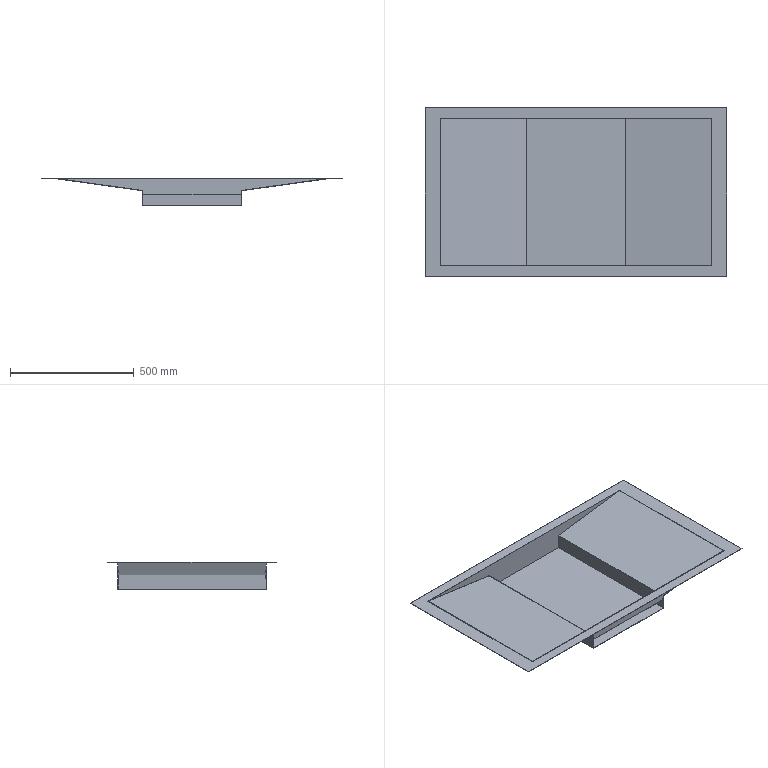Part | STEP file | HJDX-305 | 1 solid | 23 faces | box 1220 x 680 x 110 mm | volume 1513964 mm3 | plane 23
STEP:
#1=CARTESIAN_POINT('',(-200.,-300.,0.));
#2=VERTEX_POINT('',#1);
#3=CARTESIAN_POINT('',(-200.,300.,0.));
#4=VERTEX_POINT('',#3);
#5=CARTESIAN_POINT('',(-200.,0.,0.));
#6=DIRECTION('',(0.,1.,0.));
#7=VECTOR('',#6,1000.);
#8=LINE('',#5,#7);
#9=EDGE_CURVE('',#2,#4,#8,.T.);
#10=ORIENTED_EDGE('',*,*,#9,.T.);
#11=CARTESIAN_POINT('',(200.,300.,0.));
#12=VERTEX_POINT('',#11);
#13=CARTESIAN_POINT('',(0.,300.,0.));
#14=DIRECTION('',(1.,0.,0.));
#15=VECTOR('',#14,1000.);
#16=LINE('',#13,#15);
#17=EDGE_CURVE('',#4,#12,#16,.T.);
#18=ORIENTED_EDGE('',*,*,#17,.T.);
#19=CARTESIAN_POINT('',(200.,-300.,0.));
#20=VERTEX_POINT('',#19);
#21=CARTESIAN_POINT('',(200.,0.,0.));
#22=DIRECTION('',(0.,-1.,0.));
#23=VECTOR('',#22,1000.);
#24=LINE('',#21,#23);
#25=EDGE_CURVE('',#12,#20,#24,.T.);
#26=ORIENTED_EDGE('',*,*,#25,.T.);
#27=CARTESIAN_POINT('',(0.,-300.,0.));
#28=DIRECTION('',(-1.,0.,0.));
#29=VECTOR('',#28,1000.);
#30=LINE('',#27,#29);
#31=EDGE_CURVE('',#20,#2,#30,.T.);
#32=ORIENTED_EDGE('',*,*,#31,.T.);
#33=EDGE_LOOP('',(#10,#18,#26,#32));
#34=FACE_OUTER_BOUND('',#33,.T.);
#35=CARTESIAN_POINT('',(0.,0.,0.));
#36=DIRECTION('',(0.,0.,-1.));
#37=DIRECTION('',(-1.,0.,0.));
#38=AXIS2_PLACEMENT_3D('',#35,#36,#37);
#39=PLANE('',#38);
#40=ADVANCED_FACE('',(#34),#39,.T.);
#41=CARTESIAN_POINT('',(550.,300.,108.5));
#42=VERTEX_POINT('',#41);
#43=CARTESIAN_POINT('',(-550.,300.,108.5));
#44=VERTEX_POINT('',#43);
#45=CARTESIAN_POINT('',(-200.,300.,108.5));
#46=DIRECTION('',(-1.,0.,0.));
#47=VECTOR('',#46,1000.);
#48=LINE('',#45,#47);
#49=EDGE_CURVE('',#42,#44,#48,.T.);
#50=ORIENTED_EDGE('',*,*,#49,.F.);
#51=CARTESIAN_POINT('',(200.,300.,60.));
#52=VERTEX_POINT('',#51);
#53=CARTESIAN_POINT('',(200.,300.,60.));
#54=DIRECTION('',(0.9905,0.,0.1373));
#55=VECTOR('',#54,1000.);
#56=LINE('',#53,#55);
#57=EDGE_CURVE('',#52,#42,#56,.T.);
#58=ORIENTED_EDGE('',*,*,#57,.F.);
#59=CARTESIAN_POINT('',(200.,300.,60.));
#60=DIRECTION('',(0.,0.,1.));
#61=VECTOR('',#60,1000.);
#62=LINE('',#59,#61);
#63=EDGE_CURVE('',#12,#52,#62,.T.);
#64=ORIENTED_EDGE('',*,*,#63,.F.);
#65=ORIENTED_EDGE('',*,*,#17,.F.);
#66=CARTESIAN_POINT('',(-200.,300.,60.));
#67=VERTEX_POINT('',#66);
#68=CARTESIAN_POINT('',(-200.,300.,60.));
#69=DIRECTION('',(0.,0.,-1.));
#70=VECTOR('',#69,1000.);
#71=LINE('',#68,#70);
#72=EDGE_CURVE('',#67,#4,#71,.T.);
#73=ORIENTED_EDGE('',*,*,#72,.F.);
#74=CARTESIAN_POINT('',(-550.,300.,108.5));
#75=DIRECTION('',(0.9905,0.,-0.1373));
#76=VECTOR('',#75,1000.);
#77=LINE('',#74,#76);
#78=EDGE_CURVE('',#44,#67,#77,.T.);
#79=ORIENTED_EDGE('',*,*,#78,.F.);
#80=EDGE_LOOP('',(#50,#58,#64,#65,#73,#79));
#81=FACE_OUTER_BOUND('',#80,.T.);
#82=CARTESIAN_POINT('',(-200.,300.,60.));
#83=DIRECTION('',(0.,-1.,0.));
#84=DIRECTION('',(0.,0.,-1.));
#85=AXIS2_PLACEMENT_3D('',#82,#83,#84);
#86=PLANE('',#85);
#87=ADVANCED_FACE('',(#81),#86,.F.);
#88=CARTESIAN_POINT('',(-200.,-300.,60.));
#89=VERTEX_POINT('',#88);
#90=CARTESIAN_POINT('',(-200.,-300.,60.));
#91=DIRECTION('',(0.,0.,-1.));
#92=VECTOR('',#91,1000.);
#93=LINE('',#90,#92);
#94=EDGE_CURVE('',#89,#2,#93,.T.);
#95=ORIENTED_EDGE('',*,*,#94,.F.);
#96=CARTESIAN_POINT('',(-200.,-300.,60.));
#97=DIRECTION('',(0.,-1.,0.));
#98=VECTOR('',#97,1000.);
#99=LINE('',#96,#98);
#100=EDGE_CURVE('',#67,#89,#99,.T.);
#101=ORIENTED_EDGE('',*,*,#100,.F.);
#102=ORIENTED_EDGE('',*,*,#72,.T.);
#103=ORIENTED_EDGE('',*,*,#9,.F.);
#104=EDGE_LOOP('',(#95,#101,#102,#103));
#105=FACE_OUTER_BOUND('',#104,.T.);
#106=CARTESIAN_POINT('',(-200.,-300.,60.));
#107=DIRECTION('',(1.,0.,0.));
#108=DIRECTION('',(0.,0.,-1.));
#109=AXIS2_PLACEMENT_3D('',#106,#107,#108);
#110=PLANE('',#109);
#111=ADVANCED_FACE('',(#105),#110,.F.);
#112=CARTESIAN_POINT('',(-550.,-300.,108.5));
#113=VERTEX_POINT('',#112);
#114=CARTESIAN_POINT('',(550.,-300.,108.5));
#115=VERTEX_POINT('',#114);
#116=CARTESIAN_POINT('',(-200.,-300.,108.5));
#117=DIRECTION('',(1.,0.,0.));
#118=VECTOR('',#117,1000.);
#119=LINE('',#116,#118);
#120=EDGE_CURVE('',#113,#115,#119,.T.);
#121=ORIENTED_EDGE('',*,*,#120,.F.);
#122=CARTESIAN_POINT('',(-200.,-300.,60.));
#123=DIRECTION('',(-0.9905,0.,0.1373));
#124=VECTOR('',#123,1000.);
#125=LINE('',#122,#124);
#126=EDGE_CURVE('',#89,#113,#125,.T.);
#127=ORIENTED_EDGE('',*,*,#126,.F.);
#128=ORIENTED_EDGE('',*,*,#94,.T.);
#129=ORIENTED_EDGE('',*,*,#31,.F.);
#130=CARTESIAN_POINT('',(200.,-300.,60.));
#131=VERTEX_POINT('',#130);
#132=CARTESIAN_POINT('',(200.,-300.,60.));
#133=DIRECTION('',(0.,0.,-1.));
#134=VECTOR('',#133,1000.);
#135=LINE('',#132,#134);
#136=EDGE_CURVE('',#131,#20,#135,.T.);
#137=ORIENTED_EDGE('',*,*,#136,.F.);
#138=CARTESIAN_POINT('',(550.,-300.,108.5));
#139=DIRECTION('',(-0.9905,0.,-0.1373));
#140=VECTOR('',#139,1000.);
#141=LINE('',#138,#140);
#142=EDGE_CURVE('',#115,#131,#141,.T.);
#143=ORIENTED_EDGE('',*,*,#142,.F.);
#144=EDGE_LOOP('',(#121,#127,#128,#129,#137,#143));
#145=FACE_OUTER_BOUND('',#144,.T.);
#146=CARTESIAN_POINT('',(198.5,-300.,1.5));
#147=VERTEX_POINT('',#146);
#148=CARTESIAN_POINT('',(198.5,-300.,43.5));
#149=VERTEX_POINT('',#148);
#150=CARTESIAN_POINT('',(198.5,-300.,60.));
#151=DIRECTION('',(0.,0.,1.));
#152=VECTOR('',#151,1000.);
#153=LINE('',#150,#152);
#154=EDGE_CURVE('',#147,#149,#153,.T.);
#155=ORIENTED_EDGE('',*,*,#154,.F.);
#156=CARTESIAN_POINT('',(-198.5,-300.,1.5));
#157=VERTEX_POINT('',#156);
#158=CARTESIAN_POINT('',(-200.,-300.,1.5));
#159=DIRECTION('',(1.,0.,0.));
#160=VECTOR('',#159,1000.);
#161=LINE('',#158,#160);
#162=EDGE_CURVE('',#157,#147,#161,.T.);
#163=ORIENTED_EDGE('',*,*,#162,.F.);
#164=CARTESIAN_POINT('',(-198.5,-300.,43.5));
#165=VERTEX_POINT('',#164);
#166=CARTESIAN_POINT('',(-198.5,-300.,60.));
#167=DIRECTION('',(0.,0.,-1.));
#168=VECTOR('',#167,1000.);
#169=LINE('',#166,#168);
#170=EDGE_CURVE('',#165,#157,#169,.T.);
#171=ORIENTED_EDGE('',*,*,#170,.F.);
#172=CARTESIAN_POINT('',(-200.,-300.,43.5));
#173=DIRECTION('',(-1.,0.,0.));
#174=VECTOR('',#173,1000.);
#175=LINE('',#172,#174);
#176=EDGE_CURVE('',#149,#165,#175,.T.);
#177=ORIENTED_EDGE('',*,*,#176,.F.);
#178=EDGE_LOOP('',(#155,#163,#171,#177));
#179=FACE_BOUND('',#178,.T.);
#180=CARTESIAN_POINT('',(-200.,-300.,60.));
#181=DIRECTION('',(0.,1.,0.));
#182=DIRECTION('',(0.,0.,1.));
#183=AXIS2_PLACEMENT_3D('',#180,#181,#182);
#184=PLANE('',#183);
#185=ADVANCED_FACE('',(#145,#179),#184,.F.);
#186=ORIENTED_EDGE('',*,*,#63,.T.);
#187=CARTESIAN_POINT('',(200.,-300.,60.));
#188=DIRECTION('',(0.,1.,0.));
#189=VECTOR('',#188,1000.);
#190=LINE('',#187,#189);
#191=EDGE_CURVE('',#131,#52,#190,.T.);
#192=ORIENTED_EDGE('',*,*,#191,.F.);
#193=ORIENTED_EDGE('',*,*,#136,.T.);
#194=ORIENTED_EDGE('',*,*,#25,.F.);
#195=EDGE_LOOP('',(#186,#192,#193,#194));
#196=FACE_OUTER_BOUND('',#195,.T.);
#197=CARTESIAN_POINT('',(200.,-300.,60.));
#198=DIRECTION('',(-1.,0.,0.));
#199=DIRECTION('',(0.,0.,1.));
#200=AXIS2_PLACEMENT_3D('',#197,#198,#199);
#201=PLANE('',#200);
#202=ADVANCED_FACE('',(#196),#201,.F.);
#203=CARTESIAN_POINT('',(-550.,300.,108.5));
#204=DIRECTION('',(0.,-1.,0.));
#205=VECTOR('',#204,1000.);
#206=LINE('',#203,#205);
#207=EDGE_CURVE('',#44,#113,#206,.T.);
#208=ORIENTED_EDGE('',*,*,#207,.F.);
#209=ORIENTED_EDGE('',*,*,#78,.T.);
#210=ORIENTED_EDGE('',*,*,#100,.T.);
#211=ORIENTED_EDGE('',*,*,#126,.T.);
#212=EDGE_LOOP('',(#208,#209,#210,#211));
#213=FACE_OUTER_BOUND('',#212,.T.);
#214=CARTESIAN_POINT('',(-550.,300.,108.5));
#215=DIRECTION('',(0.1373,0.,0.9905));
#216=DIRECTION('',(0.9905,0.,-0.1373));
#217=AXIS2_PLACEMENT_3D('',#214,#215,#216);
#218=PLANE('',#217);
#219=ADVANCED_FACE('',(#213),#218,.F.);
#220=CARTESIAN_POINT('',(-610.,-340.,108.5));
#221=VERTEX_POINT('',#220);
#222=CARTESIAN_POINT('',(-610.,340.,108.5));
#223=VERTEX_POINT('',#222);
#224=CARTESIAN_POINT('',(-610.,0.,108.5));
#225=DIRECTION('',(0.,1.,0.));
#226=VECTOR('',#225,1000.);
#227=LINE('',#224,#226);
#228=EDGE_CURVE('',#221,#223,#227,.T.);
#229=ORIENTED_EDGE('',*,*,#228,.T.);
#230=CARTESIAN_POINT('',(610.,340.,108.5));
#231=VERTEX_POINT('',#230);
#232=CARTESIAN_POINT('',(0.,340.,108.5));
#233=DIRECTION('',(1.,0.,0.));
#234=VECTOR('',#233,1000.);
#235=LINE('',#232,#234);
#236=EDGE_CURVE('',#223,#231,#235,.T.);
#237=ORIENTED_EDGE('',*,*,#236,.T.);
#238=CARTESIAN_POINT('',(610.,-340.,108.5));
#239=VERTEX_POINT('',#238);
#240=CARTESIAN_POINT('',(610.,0.,108.5));
#241=DIRECTION('',(0.,-1.,0.));
#242=VECTOR('',#241,1000.);
#243=LINE('',#240,#242);
#244=EDGE_CURVE('',#231,#239,#243,.T.);
#245=ORIENTED_EDGE('',*,*,#244,.T.);
#246=CARTESIAN_POINT('',(0.,-340.,108.5));
#247=DIRECTION('',(-1.,0.,0.));
#248=VECTOR('',#247,1000.);
#249=LINE('',#246,#248);
#250=EDGE_CURVE('',#239,#221,#249,.T.);
#251=ORIENTED_EDGE('',*,*,#250,.T.);
#252=EDGE_LOOP('',(#229,#237,#245,#251));
#253=FACE_OUTER_BOUND('',#252,.T.);
#254=ORIENTED_EDGE('',*,*,#207,.T.);
#255=ORIENTED_EDGE('',*,*,#120,.T.);
#256=CARTESIAN_POINT('',(550.,0.,108.5));
#257=DIRECTION('',(0.,1.,0.));
#258=VECTOR('',#257,1000.);
#259=LINE('',#256,#258);
#260=EDGE_CURVE('',#115,#42,#259,.T.);
#261=ORIENTED_EDGE('',*,*,#260,.T.);
#262=ORIENTED_EDGE('',*,*,#49,.T.);
#263=EDGE_LOOP('',(#254,#255,#261,#262));
#264=FACE_BOUND('',#263,.T.);
#265=CARTESIAN_POINT('',(0.,0.,108.5));
#266=DIRECTION('',(0.,0.,-1.));
#267=DIRECTION('',(-1.,0.,0.));
#268=AXIS2_PLACEMENT_3D('',#265,#266,#267);
#269=PLANE('',#268);
#270=ADVANCED_FACE('',(#253,#264),#269,.T.);
#271=ORIENTED_EDGE('',*,*,#191,.T.);
#272=ORIENTED_EDGE('',*,*,#57,.T.);
#273=ORIENTED_EDGE('',*,*,#260,.F.);
#274=ORIENTED_EDGE('',*,*,#142,.T.);
#275=EDGE_LOOP('',(#271,#272,#273,#274));
#276=FACE_OUTER_BOUND('',#275,.T.);
#277=CARTESIAN_POINT('',(200.,300.,60.));
#278=DIRECTION('',(-0.1373,0.,0.9905));
#279=DIRECTION('',(0.9905,0.,0.1373));
#280=AXIS2_PLACEMENT_3D('',#277,#278,#279);
#281=PLANE('',#280);
#282=ADVANCED_FACE('',(#276),#281,.F.);
#283=CARTESIAN_POINT('',(198.5,-298.5,43.5));
#284=VERTEX_POINT('',#283);
#285=CARTESIAN_POINT('',(198.5,697.715,43.5));
#286=DIRECTION('',(0.,1.,0.));
#287=VECTOR('',#286,1000.);
#288=LINE('',#285,#287);
#289=EDGE_CURVE('',#149,#284,#288,.T.);
#290=ORIENTED_EDGE('',*,*,#289,.F.);
#291=ORIENTED_EDGE('',*,*,#176,.T.);
#292=CARTESIAN_POINT('',(-198.5,-298.5,43.5));
#293=VERTEX_POINT('',#292);
#294=CARTESIAN_POINT('',(-198.5,697.715,43.5));
#295=DIRECTION('',(0.,-1.,0.));
#296=VECTOR('',#295,1000.);
#297=LINE('',#294,#296);
#298=EDGE_CURVE('',#293,#165,#297,.T.);
#299=ORIENTED_EDGE('',*,*,#298,.F.);
#300=CARTESIAN_POINT('',(-198.5,-298.5,43.5));
#301=DIRECTION('',(-1.,0.,0.));
#302=VECTOR('',#301,1000.);
#303=LINE('',#300,#302);
#304=EDGE_CURVE('',#284,#293,#303,.T.);
#305=ORIENTED_EDGE('',*,*,#304,.F.);
#306=EDGE_LOOP('',(#290,#291,#299,#305));
#307=FACE_OUTER_BOUND('',#306,.T.);
#308=CARTESIAN_POINT('',(-198.5,697.715,43.5));
#309=DIRECTION('',(0.,0.,1.));
#310=DIRECTION('',(1.,0.,0.));
#311=AXIS2_PLACEMENT_3D('',#308,#309,#310);
#312=PLANE('',#311);
#313=ADVANCED_FACE('',(#307),#312,.F.);
#314=CARTESIAN_POINT('',(198.5,-298.5,61.306));
#315=VERTEX_POINT('',#314);
#316=CARTESIAN_POINT('',(198.5,-298.5,60.));
#317=DIRECTION('',(0.,0.,1.));
#318=VECTOR('',#317,1000.);
#319=LINE('',#316,#318);
#320=EDGE_CURVE('',#284,#315,#319,.T.);
#321=ORIENTED_EDGE('',*,*,#320,.T.);
#322=CARTESIAN_POINT('',(198.5,298.5,61.306));
#323=VERTEX_POINT('',#322);
#324=CARTESIAN_POINT('',(198.5,-300.,61.306));
#325=DIRECTION('',(0.,1.,0.));
#326=VECTOR('',#325,1000.);
#327=LINE('',#324,#326);
#328=EDGE_CURVE('',#315,#323,#327,.T.);
#329=ORIENTED_EDGE('',*,*,#328,.T.);
#330=CARTESIAN_POINT('',(198.5,298.5,1.5));
#331=VERTEX_POINT('',#330);
#332=CARTESIAN_POINT('',(198.5,298.5,60.));
#333=DIRECTION('',(0.,0.,-1.));
#334=VECTOR('',#333,1000.);
#335=LINE('',#332,#334);
#336=EDGE_CURVE('',#323,#331,#335,.T.);
#337=ORIENTED_EDGE('',*,*,#336,.T.);
#338=CARTESIAN_POINT('',(198.5,-300.,1.5));
#339=DIRECTION('',(0.,-1.,0.));
#340=VECTOR('',#339,1000.);
#341=LINE('',#338,#340);
#342=EDGE_CURVE('',#331,#147,#341,.T.);
#343=ORIENTED_EDGE('',*,*,#342,.T.);
#344=ORIENTED_EDGE('',*,*,#154,.T.);
#345=ORIENTED_EDGE('',*,*,#289,.T.);
#346=EDGE_LOOP('',(#321,#329,#337,#343,#344,#345));
#347=FACE_OUTER_BOUND('',#346,.T.);
#348=CARTESIAN_POINT('',(198.5,-300.,60.));
#349=DIRECTION('',(-1.,0.,0.));
#350=DIRECTION('',(0.,0.,1.));
#351=AXIS2_PLACEMENT_3D('',#348,#349,#350);
#352=PLANE('',#351);
#353=ADVANCED_FACE('',(#347),#352,.T.);
#354=CARTESIAN_POINT('',(-198.5,298.5,1.5));
#355=VERTEX_POINT('',#354);
#356=CARTESIAN_POINT('',(0.,298.5,1.5));
#357=DIRECTION('',(1.,0.,0.));
#358=VECTOR('',#357,1000.);
#359=LINE('',#356,#358);
#360=EDGE_CURVE('',#355,#331,#359,.T.);
#361=ORIENTED_EDGE('',*,*,#360,.F.);
#362=CARTESIAN_POINT('',(-198.5,0.,1.5));
#363=DIRECTION('',(0.,1.,0.));
#364=VECTOR('',#363,1000.);
#365=LINE('',#362,#364);
#366=EDGE_CURVE('',#157,#355,#365,.T.);
#367=ORIENTED_EDGE('',*,*,#366,.F.);
#368=ORIENTED_EDGE('',*,*,#162,.T.);
#369=ORIENTED_EDGE('',*,*,#342,.F.);
#370=EDGE_LOOP('',(#361,#367,#368,#369));
#371=FACE_OUTER_BOUND('',#370,.T.);
#372=CARTESIAN_POINT('',(0.,0.,1.5));
#373=DIRECTION('',(0.,0.,-1.));
#374=DIRECTION('',(-1.,0.,0.));
#375=AXIS2_PLACEMENT_3D('',#372,#373,#374);
#376=PLANE('',#375);
#377=ADVANCED_FACE('',(#371),#376,.F.);
#378=CARTESIAN_POINT('',(-198.5,298.5,61.306));
#379=VERTEX_POINT('',#378);
#380=CARTESIAN_POINT('',(-198.5,298.5,60.));
#381=DIRECTION('',(0.,0.,1.));
#382=VECTOR('',#381,1000.);
#383=LINE('',#380,#382);
#384=EDGE_CURVE('',#355,#379,#383,.T.);
#385=ORIENTED_EDGE('',*,*,#384,.T.);
#386=CARTESIAN_POINT('',(-198.5,-298.5,61.306));
#387=VERTEX_POINT('',#386);
#388=CARTESIAN_POINT('',(-198.5,-300.,61.306));
#389=DIRECTION('',(0.,-1.,0.));
#390=VECTOR('',#389,1000.);
#391=LINE('',#388,#390);
#392=EDGE_CURVE('',#379,#387,#391,.T.);
#393=ORIENTED_EDGE('',*,*,#392,.T.);
#394=CARTESIAN_POINT('',(-198.5,-298.5,60.));
#395=DIRECTION('',(0.,0.,-1.));
#396=VECTOR('',#395,1000.);
#397=LINE('',#394,#396);
#398=EDGE_CURVE('',#387,#293,#397,.T.);
#399=ORIENTED_EDGE('',*,*,#398,.T.);
#400=ORIENTED_EDGE('',*,*,#298,.T.);
#401=ORIENTED_EDGE('',*,*,#170,.T.);
#402=ORIENTED_EDGE('',*,*,#366,.T.);
#403=EDGE_LOOP('',(#385,#393,#399,#400,#401,#402));
#404=FACE_OUTER_BOUND('',#403,.T.);
#405=CARTESIAN_POINT('',(-198.5,-300.,60.));
#406=DIRECTION('',(1.,0.,0.));
#407=DIRECTION('',(0.,0.,-1.));
#408=AXIS2_PLACEMENT_3D('',#405,#406,#407);
#409=PLANE('',#408);
#410=ADVANCED_FACE('',(#404),#409,.T.);
#411=ORIENTED_EDGE('',*,*,#236,.F.);
#412=CARTESIAN_POINT('',(-610.,340.,110.));
#413=VERTEX_POINT('',#412);
#414=CARTESIAN_POINT('',(-610.,340.,108.5));
#415=DIRECTION('',(0.,0.,1.));
#416=VECTOR('',#415,1000.);
#417=LINE('',#414,#416);
#418=EDGE_CURVE('',#223,#413,#417,.T.);
#419=ORIENTED_EDGE('',*,*,#418,.T.);
#420=CARTESIAN_POINT('',(610.,340.,110.));
#421=VERTEX_POINT('',#420);
#422=CARTESIAN_POINT('',(-610.,340.,110.));
#423=DIRECTION('',(1.,0.,0.));
#424=VECTOR('',#423,1000.);
#425=LINE('',#422,#424);
#426=EDGE_CURVE('',#413,#421,#425,.T.);
#427=ORIENTED_EDGE('',*,*,#426,.T.);
#428=CARTESIAN_POINT('',(610.,340.,108.5));
#429=DIRECTION('',(0.,0.,-1.));
#430=VECTOR('',#429,1000.);
#431=LINE('',#428,#430);
#432=EDGE_CURVE('',#421,#231,#431,.T.);
#433=ORIENTED_EDGE('',*,*,#432,.T.);
#434=EDGE_LOOP('',(#411,#419,#427,#433));
#435=FACE_OUTER_BOUND('',#434,.T.);
#436=CARTESIAN_POINT('',(-610.,340.,108.5));
#437=DIRECTION('',(0.,1.,0.));
#438=DIRECTION('',(0.,0.,1.));
#439=AXIS2_PLACEMENT_3D('',#436,#437,#438);
#440=PLANE('',#439);
#441=ADVANCED_FACE('',(#435),#440,.T.);
#442=ORIENTED_EDGE('',*,*,#228,.F.);
#443=CARTESIAN_POINT('',(-610.,-340.,110.));
#444=VERTEX_POINT('',#443);
#445=CARTESIAN_POINT('',(-610.,-340.,108.5));
#446=DIRECTION('',(0.,0.,1.));
#447=VECTOR('',#446,1000.);
#448=LINE('',#445,#447);
#449=EDGE_CURVE('',#221,#444,#448,.T.);
#450=ORIENTED_EDGE('',*,*,#449,.T.);
#451=CARTESIAN_POINT('',(-610.,-340.,110.));
#452=DIRECTION('',(0.,1.,0.));
#453=VECTOR('',#452,1000.);
#454=LINE('',#451,#453);
#455=EDGE_CURVE('',#444,#413,#454,.T.);
#456=ORIENTED_EDGE('',*,*,#455,.T.);
#457=ORIENTED_EDGE('',*,*,#418,.F.);
#458=EDGE_LOOP('',(#442,#450,#456,#457));
#459=FACE_OUTER_BOUND('',#458,.T.);
#460=CARTESIAN_POINT('',(-610.,-340.,108.5));
#461=DIRECTION('',(-1.,0.,0.));
#462=DIRECTION('',(0.,0.,1.));
#463=AXIS2_PLACEMENT_3D('',#460,#461,#462);
#464=PLANE('',#463);
#465=ADVANCED_FACE('',(#459),#464,.T.);
#466=ORIENTED_EDGE('',*,*,#250,.F.);
#467=CARTESIAN_POINT('',(610.,-340.,110.));
#468=VERTEX_POINT('',#467);
#469=CARTESIAN_POINT('',(610.,-340.,108.5));
#470=DIRECTION('',(0.,0.,1.));
#471=VECTOR('',#470,1000.);
#472=LINE('',#469,#471);
#473=EDGE_CURVE('',#239,#468,#472,.T.);
#474=ORIENTED_EDGE('',*,*,#473,.T.);
#475=CARTESIAN_POINT('',(-610.,-340.,110.));
#476=DIRECTION('',(-1.,0.,0.));
#477=VECTOR('',#476,1000.);
#478=LINE('',#475,#477);
#479=EDGE_CURVE('',#468,#444,#478,.T.);
#480=ORIENTED_EDGE('',*,*,#479,.T.);
#481=ORIENTED_EDGE('',*,*,#449,.F.);
#482=EDGE_LOOP('',(#466,#474,#480,#481));
#483=FACE_OUTER_BOUND('',#482,.T.);
#484=CARTESIAN_POINT('',(-610.,-340.,108.5));
#485=DIRECTION('',(0.,-1.,0.));
#486=DIRECTION('',(0.,0.,-1.));
#487=AXIS2_PLACEMENT_3D('',#484,#485,#486);
#488=PLANE('',#487);
#489=ADVANCED_FACE('',(#483),#488,.T.);
#490=ORIENTED_EDGE('',*,*,#244,.F.);
#491=ORIENTED_EDGE('',*,*,#432,.F.);
#492=CARTESIAN_POINT('',(610.,-340.,110.));
#493=DIRECTION('',(0.,-1.,0.));
#494=VECTOR('',#493,1000.);
#495=LINE('',#492,#494);
#496=EDGE_CURVE('',#421,#468,#495,.T.);
#497=ORIENTED_EDGE('',*,*,#496,.T.);
#498=ORIENTED_EDGE('',*,*,#473,.F.);
#499=EDGE_LOOP('',(#490,#491,#497,#498));
#500=FACE_OUTER_BOUND('',#499,.T.);
#501=CARTESIAN_POINT('',(610.,-340.,108.5));
#502=DIRECTION('',(1.,0.,0.));
#503=DIRECTION('',(0.,0.,-1.));
#504=AXIS2_PLACEMENT_3D('',#501,#502,#503);
#505=PLANE('',#504);
#506=ADVANCED_FACE('',(#500),#505,.T.);
#507=CARTESIAN_POINT('',(548.5,-298.5,109.806));
#508=VERTEX_POINT('',#507);
#509=CARTESIAN_POINT('',(548.5,-298.5,109.806));
#510=DIRECTION('',(-0.9905,0.,-0.1373));
#511=VECTOR('',#510,1000.);
#512=LINE('',#509,#511);
#513=EDGE_CURVE('',#508,#315,#512,.T.);
#514=ORIENTED_EDGE('',*,*,#513,.T.);
#515=ORIENTED_EDGE('',*,*,#320,.F.);
#516=ORIENTED_EDGE('',*,*,#304,.T.);
#517=ORIENTED_EDGE('',*,*,#398,.F.);
#518=CARTESIAN_POINT('',(-548.5,-298.5,109.806));
#519=VERTEX_POINT('',#518);
#520=CARTESIAN_POINT('',(-198.5,-298.5,61.306));
#521=DIRECTION('',(-0.9905,0.,0.1373));
#522=VECTOR('',#521,1000.);
#523=LINE('',#520,#522);
#524=EDGE_CURVE('',#387,#519,#523,.T.);
#525=ORIENTED_EDGE('',*,*,#524,.T.);
#526=CARTESIAN_POINT('',(-548.5,-298.5,110.));
#527=VERTEX_POINT('',#526);
#528=CARTESIAN_POINT('',(-548.5,-298.5,110.));
#529=DIRECTION('',(0.,0.,-1.));
#530=VECTOR('',#529,1000.);
#531=LINE('',#528,#530);
#532=EDGE_CURVE('',#527,#519,#531,.T.);
#533=ORIENTED_EDGE('',*,*,#532,.F.);
#534=CARTESIAN_POINT('',(548.5,-298.5,110.));
#535=VERTEX_POINT('',#534);
#536=CARTESIAN_POINT('',(-200.,-298.5,110.));
#537=DIRECTION('',(1.,0.,0.));
#538=VECTOR('',#537,1000.);
#539=LINE('',#536,#538);
#540=EDGE_CURVE('',#527,#535,#539,.T.);
#541=ORIENTED_EDGE('',*,*,#540,.T.);
#542=CARTESIAN_POINT('',(548.5,-298.5,110.));
#543=DIRECTION('',(0.,0.,1.));
#544=VECTOR('',#543,1000.);
#545=LINE('',#542,#544);
#546=EDGE_CURVE('',#508,#535,#545,.T.);
#547=ORIENTED_EDGE('',*,*,#546,.F.);
#548=EDGE_LOOP('',(#514,#515,#516,#517,#525,#533,#541,#547));
#549=FACE_OUTER_BOUND('',#548,.T.);
#550=CARTESIAN_POINT('',(-200.,-298.5,60.));
#551=DIRECTION('',(0.,1.,0.));
#552=DIRECTION('',(0.,0.,1.));
#553=AXIS2_PLACEMENT_3D('',#550,#551,#552);
#554=PLANE('',#553);
#555=ADVANCED_FACE('',(#549),#554,.T.);
#556=CARTESIAN_POINT('',(548.5,298.5,109.806));
#557=VERTEX_POINT('',#556);
#558=CARTESIAN_POINT('',(199.794,298.5,61.486));
#559=DIRECTION('',(-0.9905,0.,-0.1373));
#560=VECTOR('',#559,1000.);
#561=LINE('',#558,#560);
#562=EDGE_CURVE('',#557,#323,#561,.T.);
#563=ORIENTED_EDGE('',*,*,#562,.T.);
#564=ORIENTED_EDGE('',*,*,#328,.F.);
#565=ORIENTED_EDGE('',*,*,#513,.F.);
#566=CARTESIAN_POINT('',(548.5,300.,109.806));
#567=DIRECTION('',(0.,1.,0.));
#568=VECTOR('',#567,1000.);
#569=LINE('',#566,#568);
#570=EDGE_CURVE('',#508,#557,#569,.T.);
#571=ORIENTED_EDGE('',*,*,#570,.T.);
#572=EDGE_LOOP('',(#563,#564,#565,#571));
#573=FACE_OUTER_BOUND('',#572,.T.);
#574=CARTESIAN_POINT('',(199.794,300.,61.486));
#575=DIRECTION('',(-0.1373,0.,0.9905));
#576=DIRECTION('',(0.9905,0.,0.1373));
#577=AXIS2_PLACEMENT_3D('',#574,#575,#576);
#578=PLANE('',#577);
#579=ADVANCED_FACE('',(#573),#578,.T.);
#580=CARTESIAN_POINT('',(-548.5,298.5,109.806));
#581=VERTEX_POINT('',#580);
#582=CARTESIAN_POINT('',(-548.5,298.5,110.));
#583=VERTEX_POINT('',#582);
#584=CARTESIAN_POINT('',(-548.5,298.5,110.));
#585=DIRECTION('',(0.,0.,1.));
#586=VECTOR('',#585,1000.);
#587=LINE('',#584,#586);
#588=EDGE_CURVE('',#581,#583,#587,.T.);
#589=ORIENTED_EDGE('',*,*,#588,.F.);
#590=CARTESIAN_POINT('',(-548.5,298.5,109.806));
#591=DIRECTION('',(0.9905,0.,-0.1373));
#592=VECTOR('',#591,1000.);
#593=LINE('',#590,#592);
#594=EDGE_CURVE('',#581,#379,#593,.T.);
#595=ORIENTED_EDGE('',*,*,#594,.T.);
#596=ORIENTED_EDGE('',*,*,#384,.F.);
#597=ORIENTED_EDGE('',*,*,#360,.T.);
#598=ORIENTED_EDGE('',*,*,#336,.F.);
#599=ORIENTED_EDGE('',*,*,#562,.F.);
#600=CARTESIAN_POINT('',(548.5,298.5,110.));
#601=VERTEX_POINT('',#600);
#602=CARTESIAN_POINT('',(548.5,298.5,60.));
#603=DIRECTION('',(0.,0.,1.));
#604=VECTOR('',#603,1000.);
#605=LINE('',#602,#604);
#606=EDGE_CURVE('',#557,#601,#605,.T.);
#607=ORIENTED_EDGE('',*,*,#606,.T.);
#608=CARTESIAN_POINT('',(-200.,298.5,110.));
#609=DIRECTION('',(-1.,0.,0.));
#610=VECTOR('',#609,1000.);
#611=LINE('',#608,#610);
#612=EDGE_CURVE('',#601,#583,#611,.T.);
#613=ORIENTED_EDGE('',*,*,#612,.T.);
#614=EDGE_LOOP('',(#589,#595,#596,#597,#598,#599,#607,#613));
#615=FACE_OUTER_BOUND('',#614,.T.);
#616=CARTESIAN_POINT('',(-200.,298.5,60.));
#617=DIRECTION('',(0.,-1.,0.));
#618=DIRECTION('',(0.,0.,-1.));
#619=AXIS2_PLACEMENT_3D('',#616,#617,#618);
#620=PLANE('',#619);
#621=ADVANCED_FACE('',(#615),#620,.T.);
#622=ORIENTED_EDGE('',*,*,#594,.F.);
#623=CARTESIAN_POINT('',(-548.5,300.,109.806));
#624=DIRECTION('',(0.,-1.,0.));
#625=VECTOR('',#624,1000.);
#626=LINE('',#623,#625);
#627=EDGE_CURVE('',#581,#519,#626,.T.);
#628=ORIENTED_EDGE('',*,*,#627,.T.);
#629=ORIENTED_EDGE('',*,*,#524,.F.);
#630=ORIENTED_EDGE('',*,*,#392,.F.);
#631=EDGE_LOOP('',(#622,#628,#629,#630));
#632=FACE_OUTER_BOUND('',#631,.T.);
#633=CARTESIAN_POINT('',(-549.794,300.,109.986));
#634=DIRECTION('',(0.1373,0.,0.9905));
#635=DIRECTION('',(0.9905,0.,-0.1373));
#636=AXIS2_PLACEMENT_3D('',#633,#634,#635);
#637=PLANE('',#636);
#638=ADVANCED_FACE('',(#632),#637,.T.);
#639=ORIENTED_EDGE('',*,*,#426,.F.);
#640=ORIENTED_EDGE('',*,*,#455,.F.);
#641=ORIENTED_EDGE('',*,*,#479,.F.);
#642=ORIENTED_EDGE('',*,*,#496,.F.);
#643=EDGE_LOOP('',(#639,#640,#641,#642));
#644=FACE_OUTER_BOUND('',#643,.T.);
#645=ORIENTED_EDGE('',*,*,#540,.F.);
#646=CARTESIAN_POINT('',(-548.5,0.,110.));
#647=DIRECTION('',(0.,-1.,0.));
#648=VECTOR('',#647,1000.);
#649=LINE('',#646,#648);
#650=EDGE_CURVE('',#583,#527,#649,.T.);
#651=ORIENTED_EDGE('',*,*,#650,.F.);
#652=ORIENTED_EDGE('',*,*,#612,.F.);
#653=CARTESIAN_POINT('',(548.5,0.,110.));
#654=DIRECTION('',(0.,1.,0.));
#655=VECTOR('',#654,1000.);
#656=LINE('',#653,#655);
#657=EDGE_CURVE('',#535,#601,#656,.T.);
#658=ORIENTED_EDGE('',*,*,#657,.F.);
#659=EDGE_LOOP('',(#645,#651,#652,#658));
#660=FACE_BOUND('',#659,.T.);
#661=CARTESIAN_POINT('',(0.,0.,110.));
#662=DIRECTION('',(0.,0.,-1.));
#663=DIRECTION('',(-1.,0.,0.));
#664=AXIS2_PLACEMENT_3D('',#661,#662,#663);
#665=PLANE('',#664);
#666=ADVANCED_FACE('',(#644,#660),#665,.F.);
#667=ORIENTED_EDGE('',*,*,#606,.F.);
#668=ORIENTED_EDGE('',*,*,#570,.F.);
#669=ORIENTED_EDGE('',*,*,#546,.T.);
#670=ORIENTED_EDGE('',*,*,#657,.T.);
#671=EDGE_LOOP('',(#667,#668,#669,#670));
#672=FACE_OUTER_BOUND('',#671,.T.);
#673=CARTESIAN_POINT('',(548.5,-300.,110.));
#674=DIRECTION('',(-1.,0.,0.));
#675=DIRECTION('',(0.,0.,1.));
#676=AXIS2_PLACEMENT_3D('',#673,#674,#675);
#677=PLANE('',#676);
#678=ADVANCED_FACE('',(#672),#677,.T.);
#679=ORIENTED_EDGE('',*,*,#532,.T.);
#680=ORIENTED_EDGE('',*,*,#627,.F.);
#681=ORIENTED_EDGE('',*,*,#588,.T.);
#682=ORIENTED_EDGE('',*,*,#650,.T.);
#683=EDGE_LOOP('',(#679,#680,#681,#682));
#684=FACE_OUTER_BOUND('',#683,.T.);
#685=CARTESIAN_POINT('',(-548.5,-300.,110.));
#686=DIRECTION('',(1.,0.,0.));
#687=DIRECTION('',(0.,0.,-1.));
#688=AXIS2_PLACEMENT_3D('',#685,#686,#687);
#689=PLANE('',#688);
#690=ADVANCED_FACE('',(#684),#689,.T.);
#691=CLOSED_SHELL('',(#40,#87,#111,#185,#202,#219,#270,#282,#313,#353,#377,#410,#441,#465,#489,#506,#555,#579,#621,#638,#666,#678,#690));
#692=MANIFOLD_SOLID_BREP('',#691);
#693=CARTESIAN_POINT('',(0.,0.,0.));
#694=DIRECTION('',(0.,0.,1.));
#695=DIRECTION('',(1.,0.,0.));
#696=AXIS2_PLACEMENT_3D('',#693,#694,#695);
#697=(LENGTH_UNIT()NAMED_UNIT(*)SI_UNIT(.MILLI.,.METRE.));
#698=UNCERTAINTY_MEASURE_WITH_UNIT(LENGTH_MEASURE(0.00001),#697,'','');
#699=(NAMED_UNIT(*)PLANE_ANGLE_UNIT()SI_UNIT($,.RADIAN.));
#700=(NAMED_UNIT(*)SI_UNIT($,.STERADIAN.)SOLID_ANGLE_UNIT());
#701=(GEOMETRIC_REPRESENTATION_CONTEXT(3)GLOBAL_UNCERTAINTY_ASSIGNED_CONTEXT((#698))GLOBAL_UNIT_ASSIGNED_CONTEXT((#697,#699,#700))REPRESENTATION_CONTEXT('',''));
#702=ADVANCED_BREP_SHAPE_REPRESENTATION('',(#692,#696),#701);